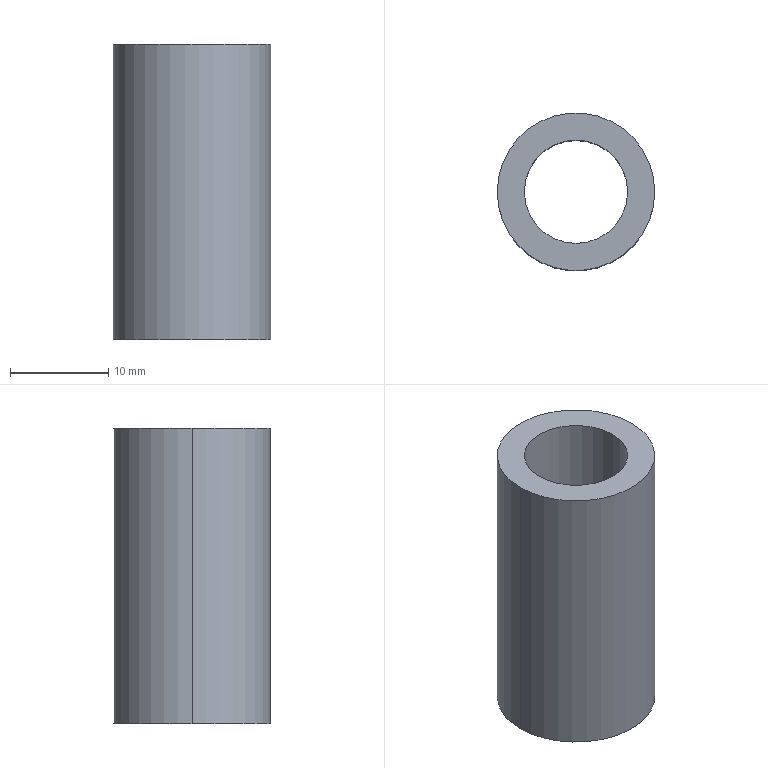Part | SolidWorks | features Extrusion 1, HoleWzd 1 | 1 solid | 6 faces | box 16 x 16 x 30 mm | volume 3434 mm3 | cylinder 4 | plane 2 | commonest cylinder face diameters 10.5 x2 16 x2
STEP:
#1=CARTESIAN_POINT('',(-5.25,0.,0.));
#2=VERTEX_POINT('',#1);
#3=CARTESIAN_POINT('',(5.25,0.,0.));
#4=VERTEX_POINT('',#3);
#5=CARTESIAN_POINT('',(0.,0.,0.));
#6=DIRECTION('',(0.,0.,1.));
#7=DIRECTION('',(1.,0.,0.));
#8=AXIS2_PLACEMENT_3D('',#5,#6,#7);
#9=CIRCLE('',#8,5.25);
#10=EDGE_CURVE('',#2,#4,#9,.T.);
#11=ORIENTED_EDGE('',*,*,#10,.F.);
#12=CARTESIAN_POINT('',(-5.25,0.,30.));
#13=VERTEX_POINT('',#12);
#14=CARTESIAN_POINT('',(-5.25,0.,30.));
#15=DIRECTION('',(0.,0.,1.));
#16=VECTOR('',#15,1000.);
#17=LINE('',#14,#16);
#18=EDGE_CURVE('',#2,#13,#17,.T.);
#19=ORIENTED_EDGE('',*,*,#18,.T.);
#20=CARTESIAN_POINT('',(5.25,0.,30.));
#21=VERTEX_POINT('',#20);
#22=CARTESIAN_POINT('',(0.,0.,30.));
#23=DIRECTION('',(0.,0.,1.));
#24=DIRECTION('',(1.,0.,0.));
#25=AXIS2_PLACEMENT_3D('',#22,#23,#24);
#26=CIRCLE('',#25,5.25);
#27=EDGE_CURVE('',#13,#21,#26,.T.);
#28=ORIENTED_EDGE('',*,*,#27,.T.);
#29=CARTESIAN_POINT('',(5.25,0.,30.));
#30=DIRECTION('',(0.,0.,1.));
#31=VECTOR('',#30,1000.);
#32=LINE('',#29,#31);
#33=EDGE_CURVE('',#4,#21,#32,.T.);
#34=ORIENTED_EDGE('',*,*,#33,.F.);
#35=EDGE_LOOP('',(#11,#19,#28,#34));
#36=FACE_OUTER_BOUND('',#35,.T.);
#37=CARTESIAN_POINT('',(0.,0.,30.));
#38=DIRECTION('',(0.,0.,1.));
#39=DIRECTION('',(1.,0.,0.));
#40=AXIS2_PLACEMENT_3D('',#37,#38,#39);
#41=CYLINDRICAL_SURFACE('',#40,5.25);
#42=ADVANCED_FACE('',(#36),#41,.F.);
#43=CARTESIAN_POINT('',(8.,0.,30.));
#44=VERTEX_POINT('',#43);
#45=CARTESIAN_POINT('',(-8.,0.,30.));
#46=VERTEX_POINT('',#45);
#47=CARTESIAN_POINT('',(0.,0.,30.));
#48=DIRECTION('',(0.,0.,1.));
#49=DIRECTION('',(1.,0.,0.));
#50=AXIS2_PLACEMENT_3D('',#47,#48,#49);
#51=CIRCLE('',#50,8.);
#52=EDGE_CURVE('',#44,#46,#51,.T.);
#53=ORIENTED_EDGE('',*,*,#52,.F.);
#54=CARTESIAN_POINT('',(8.,0.,0.));
#55=VERTEX_POINT('',#54);
#56=CARTESIAN_POINT('',(8.,0.,30.));
#57=DIRECTION('',(0.,0.,-1.));
#58=VECTOR('',#57,1000.);
#59=LINE('',#56,#58);
#60=EDGE_CURVE('',#44,#55,#59,.T.);
#61=ORIENTED_EDGE('',*,*,#60,.T.);
#62=CARTESIAN_POINT('',(-8.,0.,0.));
#63=VERTEX_POINT('',#62);
#64=CARTESIAN_POINT('',(0.,0.,0.));
#65=DIRECTION('',(0.,0.,1.));
#66=DIRECTION('',(1.,0.,0.));
#67=AXIS2_PLACEMENT_3D('',#64,#65,#66);
#68=CIRCLE('',#67,8.);
#69=EDGE_CURVE('',#55,#63,#68,.T.);
#70=ORIENTED_EDGE('',*,*,#69,.T.);
#71=CARTESIAN_POINT('',(-8.,0.,30.));
#72=DIRECTION('',(0.,0.,-1.));
#73=VECTOR('',#72,1000.);
#74=LINE('',#71,#73);
#75=EDGE_CURVE('',#46,#63,#74,.T.);
#76=ORIENTED_EDGE('',*,*,#75,.F.);
#77=EDGE_LOOP('',(#53,#61,#70,#76));
#78=FACE_OUTER_BOUND('',#77,.T.);
#79=CARTESIAN_POINT('',(0.,0.,30.));
#80=DIRECTION('',(0.,0.,-1.));
#81=DIRECTION('',(-1.,0.,0.));
#82=AXIS2_PLACEMENT_3D('',#79,#80,#81);
#83=CYLINDRICAL_SURFACE('',#82,8.);
#84=ADVANCED_FACE('',(#78),#83,.T.);
#85=ORIENTED_EDGE('',*,*,#60,.F.);
#86=CARTESIAN_POINT('',(0.,0.,30.));
#87=DIRECTION('',(0.,0.,1.));
#88=DIRECTION('',(1.,0.,0.));
#89=AXIS2_PLACEMENT_3D('',#86,#87,#88);
#90=CIRCLE('',#89,8.);
#91=EDGE_CURVE('',#46,#44,#90,.T.);
#92=ORIENTED_EDGE('',*,*,#91,.F.);
#93=ORIENTED_EDGE('',*,*,#75,.T.);
#94=CARTESIAN_POINT('',(0.,0.,0.));
#95=DIRECTION('',(0.,0.,1.));
#96=DIRECTION('',(1.,0.,0.));
#97=AXIS2_PLACEMENT_3D('',#94,#95,#96);
#98=CIRCLE('',#97,8.);
#99=EDGE_CURVE('',#63,#55,#98,.T.);
#100=ORIENTED_EDGE('',*,*,#99,.T.);
#101=EDGE_LOOP('',(#85,#92,#93,#100));
#102=FACE_OUTER_BOUND('',#101,.T.);
#103=CARTESIAN_POINT('',(0.,0.,30.));
#104=DIRECTION('',(0.,0.,-1.));
#105=DIRECTION('',(-1.,0.,0.));
#106=AXIS2_PLACEMENT_3D('',#103,#104,#105);
#107=CYLINDRICAL_SURFACE('',#106,8.);
#108=ADVANCED_FACE('',(#102),#107,.T.);
#109=CARTESIAN_POINT('',(0.,0.,30.));
#110=DIRECTION('',(0.,0.,1.));
#111=DIRECTION('',(1.,0.,0.));
#112=AXIS2_PLACEMENT_3D('',#109,#110,#111);
#113=CIRCLE('',#112,5.25);
#114=EDGE_CURVE('',#21,#13,#113,.T.);
#115=ORIENTED_EDGE('',*,*,#114,.F.);
#116=ORIENTED_EDGE('',*,*,#27,.F.);
#117=EDGE_LOOP('',(#115,#116));
#118=FACE_BOUND('',#117,.T.);
#119=ORIENTED_EDGE('',*,*,#91,.T.);
#120=ORIENTED_EDGE('',*,*,#52,.T.);
#121=EDGE_LOOP('',(#119,#120));
#122=FACE_OUTER_BOUND('',#121,.T.);
#123=CARTESIAN_POINT('',(0.,0.,30.));
#124=DIRECTION('',(0.,0.,1.));
#125=DIRECTION('',(1.,0.,0.));
#126=AXIS2_PLACEMENT_3D('',#123,#124,#125);
#127=PLANE('',#126);
#128=ADVANCED_FACE('',(#118,#122),#127,.T.);
#129=CARTESIAN_POINT('',(0.,0.,0.));
#130=DIRECTION('',(0.,0.,1.));
#131=DIRECTION('',(1.,0.,0.));
#132=AXIS2_PLACEMENT_3D('',#129,#130,#131);
#133=CIRCLE('',#132,5.25);
#134=EDGE_CURVE('',#4,#2,#133,.T.);
#135=ORIENTED_EDGE('',*,*,#134,.T.);
#136=ORIENTED_EDGE('',*,*,#10,.T.);
#137=EDGE_LOOP('',(#135,#136));
#138=FACE_BOUND('',#137,.T.);
#139=ORIENTED_EDGE('',*,*,#99,.F.);
#140=ORIENTED_EDGE('',*,*,#69,.F.);
#141=EDGE_LOOP('',(#139,#140));
#142=FACE_OUTER_BOUND('',#141,.T.);
#143=CARTESIAN_POINT('',(0.,0.,0.));
#144=DIRECTION('',(0.,0.,1.));
#145=DIRECTION('',(1.,0.,0.));
#146=AXIS2_PLACEMENT_3D('',#143,#144,#145);
#147=PLANE('',#146);
#148=ADVANCED_FACE('',(#138,#142),#147,.F.);
#149=ORIENTED_EDGE('',*,*,#18,.F.);
#150=ORIENTED_EDGE('',*,*,#134,.F.);
#151=ORIENTED_EDGE('',*,*,#33,.T.);
#152=ORIENTED_EDGE('',*,*,#114,.T.);
#153=EDGE_LOOP('',(#149,#150,#151,#152));
#154=FACE_OUTER_BOUND('',#153,.T.);
#155=CARTESIAN_POINT('',(0.,0.,30.));
#156=DIRECTION('',(0.,0.,1.));
#157=DIRECTION('',(1.,0.,0.));
#158=AXIS2_PLACEMENT_3D('',#155,#156,#157);
#159=CYLINDRICAL_SURFACE('',#158,5.25);
#160=ADVANCED_FACE('',(#154),#159,.F.);
#161=CLOSED_SHELL('',(#42,#84,#108,#128,#148,#160));
#162=MANIFOLD_SOLID_BREP('',#161);
#163=CARTESIAN_POINT('',(0.,0.,0.));
#164=DIRECTION('',(0.,0.,1.));
#165=DIRECTION('',(1.,0.,0.));
#166=AXIS2_PLACEMENT_3D('',#163,#164,#165);
#167=(LENGTH_UNIT()NAMED_UNIT(*)SI_UNIT(.MILLI.,.METRE.));
#168=UNCERTAINTY_MEASURE_WITH_UNIT(LENGTH_MEASURE(0.00001),#167,'','');
#169=(NAMED_UNIT(*)PLANE_ANGLE_UNIT()SI_UNIT($,.RADIAN.));
#170=(NAMED_UNIT(*)SI_UNIT($,.STERADIAN.)SOLID_ANGLE_UNIT());
#171=(GEOMETRIC_REPRESENTATION_CONTEXT(3)GLOBAL_UNCERTAINTY_ASSIGNED_CONTEXT((#168))GLOBAL_UNIT_ASSIGNED_CONTEXT((#167,#169,#170))REPRESENTATION_CONTEXT('',''));
#172=ADVANCED_BREP_SHAPE_REPRESENTATION('',(#162,#166),#171);